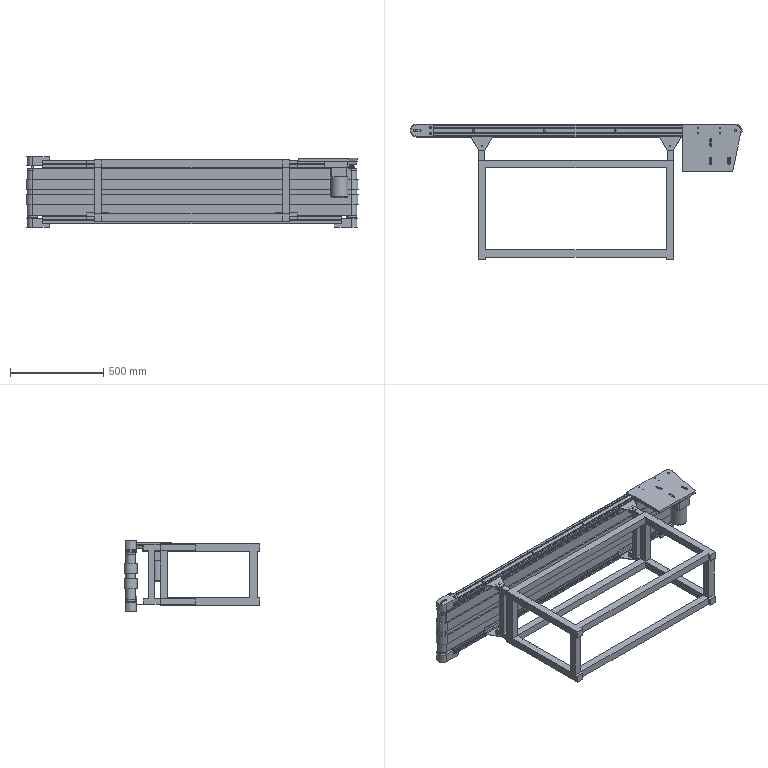Part | NX | 19 solids | 585 faces | box 1780 x 728 x 380 mm | volume 26797017 mm3 | plane 390 | cylinder 193 | torus 1 | cone 1 | commonest cylinder face diameters 3 x41 10 x31 6.5 x23 12 x12 5 x10 50 x9